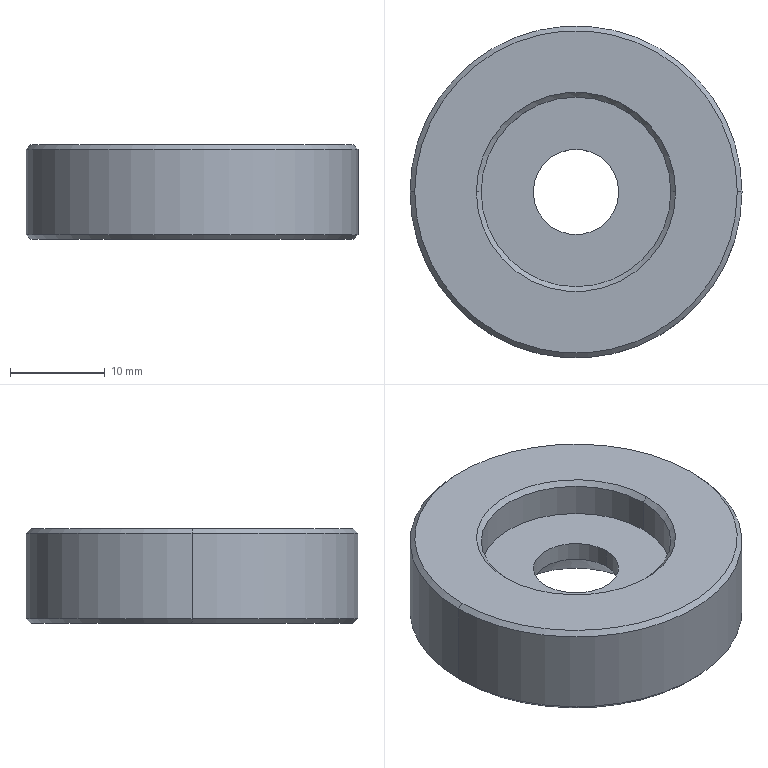Part | SolidWorks | features Chamfer 2, Extrusion 1, HoleWzd 1, ICE 1 | 1 solid | 17 faces | box 35 x 35 x 10 mm | volume 7654 mm3 | cone 8 | cylinder 6 | plane 3 | commonest cylinder face diameters 9 x2 20 x2 35 x2
STEP:
#1=CARTESIAN_POINT('',(-10.,0.,9.5));
#2=VERTEX_POINT('',#1);
#3=CARTESIAN_POINT('',(10.,0.,9.5));
#4=VERTEX_POINT('',#3);
#5=CARTESIAN_POINT('',(0.,0.,9.5));
#6=DIRECTION('',(0.,0.,1.));
#7=DIRECTION('',(1.,0.,0.));
#8=AXIS2_PLACEMENT_3D('',#5,#6,#7);
#9=CIRCLE('',#8,10.);
#10=EDGE_CURVE('',#2,#4,#9,.T.);
#11=ORIENTED_EDGE('',*,*,#10,.F.);
#12=CARTESIAN_POINT('',(-10.5,0.,10.));
#13=VERTEX_POINT('',#12);
#14=CARTESIAN_POINT('',(-10.,0.,9.5));
#15=DIRECTION('',(-0.7071,0.,0.7071));
#16=VECTOR('',#15,1000.);
#17=LINE('',#14,#16);
#18=EDGE_CURVE('',#2,#13,#17,.T.);
#19=ORIENTED_EDGE('',*,*,#18,.T.);
#20=CARTESIAN_POINT('',(10.5,0.,10.));
#21=VERTEX_POINT('',#20);
#22=CARTESIAN_POINT('',(0.,0.,10.));
#23=DIRECTION('',(0.,0.,-1.));
#24=DIRECTION('',(1.,0.,0.));
#25=AXIS2_PLACEMENT_3D('',#22,#23,#24);
#26=CIRCLE('',#25,10.5);
#27=EDGE_CURVE('',#21,#13,#26,.T.);
#28=ORIENTED_EDGE('',*,*,#27,.F.);
#29=CARTESIAN_POINT('',(10.,0.,9.5));
#30=DIRECTION('',(0.7071,0.,0.7071));
#31=VECTOR('',#30,1000.);
#32=LINE('',#29,#31);
#33=EDGE_CURVE('',#4,#21,#32,.T.);
#34=ORIENTED_EDGE('',*,*,#33,.F.);
#35=EDGE_LOOP('',(#11,#19,#28,#34));
#36=FACE_OUTER_BOUND('',#35,.T.);
#37=CARTESIAN_POINT('',(0.,0.,9.5));
#38=DIRECTION('',(0.,0.,1.));
#39=DIRECTION('',(1.,0.,0.));
#40=AXIS2_PLACEMENT_3D('',#37,#38,#39);
#41=CONICAL_SURFACE('',#40,10.,0.7854);
#42=ADVANCED_FACE('',(#36),#41,.F.);
#43=CARTESIAN_POINT('',(-10.,0.,6.));
#44=VERTEX_POINT('',#43);
#45=CARTESIAN_POINT('',(10.,0.,6.));
#46=VERTEX_POINT('',#45);
#47=CARTESIAN_POINT('',(0.,0.,6.));
#48=DIRECTION('',(0.,0.,1.));
#49=DIRECTION('',(1.,0.,0.));
#50=AXIS2_PLACEMENT_3D('',#47,#48,#49);
#51=CIRCLE('',#50,10.);
#52=EDGE_CURVE('',#44,#46,#51,.T.);
#53=ORIENTED_EDGE('',*,*,#52,.F.);
#54=CARTESIAN_POINT('',(-10.,0.,6.));
#55=DIRECTION('',(0.,0.,1.));
#56=VECTOR('',#55,1000.);
#57=LINE('',#54,#56);
#58=EDGE_CURVE('',#44,#2,#57,.T.);
#59=ORIENTED_EDGE('',*,*,#58,.T.);
#60=ORIENTED_EDGE('',*,*,#10,.T.);
#61=CARTESIAN_POINT('',(10.,0.,6.));
#62=DIRECTION('',(0.,0.,1.));
#63=VECTOR('',#62,1000.);
#64=LINE('',#61,#63);
#65=EDGE_CURVE('',#46,#4,#64,.T.);
#66=ORIENTED_EDGE('',*,*,#65,.F.);
#67=EDGE_LOOP('',(#53,#59,#60,#66));
#68=FACE_OUTER_BOUND('',#67,.T.);
#69=CARTESIAN_POINT('',(0.,0.,6.));
#70=DIRECTION('',(0.,0.,1.));
#71=DIRECTION('',(1.,0.,0.));
#72=AXIS2_PLACEMENT_3D('',#69,#70,#71);
#73=CYLINDRICAL_SURFACE('',#72,10.);
#74=ADVANCED_FACE('',(#68),#73,.F.);
#75=CARTESIAN_POINT('',(4.5,0.,4.));
#76=VERTEX_POINT('',#75);
#77=CARTESIAN_POINT('',(-4.5,0.,4.));
#78=VERTEX_POINT('',#77);
#79=CARTESIAN_POINT('',(0.,0.,4.));
#80=DIRECTION('',(0.,0.,-1.));
#81=DIRECTION('',(-1.,0.,0.));
#82=AXIS2_PLACEMENT_3D('',#79,#80,#81);
#83=CIRCLE('',#82,4.5);
#84=EDGE_CURVE('',#76,#78,#83,.T.);
#85=ORIENTED_EDGE('',*,*,#84,.F.);
#86=CARTESIAN_POINT('',(8.5,0.,0.));
#87=VERTEX_POINT('',#86);
#88=CARTESIAN_POINT('',(8.5,0.,0.));
#89=DIRECTION('',(0.7071,0.,-0.7071));
#90=VECTOR('',#89,1000.);
#91=LINE('',#88,#90);
#92=EDGE_CURVE('',#76,#87,#91,.T.);
#93=ORIENTED_EDGE('',*,*,#92,.T.);
#94=CARTESIAN_POINT('',(-8.5,0.,0.));
#95=VERTEX_POINT('',#94);
#96=CARTESIAN_POINT('',(0.,0.,0.));
#97=DIRECTION('',(0.,0.,-1.));
#98=DIRECTION('',(-1.,0.,0.));
#99=AXIS2_PLACEMENT_3D('',#96,#97,#98);
#100=CIRCLE('',#99,8.5);
#101=EDGE_CURVE('',#87,#95,#100,.T.);
#102=ORIENTED_EDGE('',*,*,#101,.T.);
#103=CARTESIAN_POINT('',(-8.5,0.,0.));
#104=DIRECTION('',(-0.7071,0.,-0.7071));
#105=VECTOR('',#104,1000.);
#106=LINE('',#103,#105);
#107=EDGE_CURVE('',#78,#95,#106,.T.);
#108=ORIENTED_EDGE('',*,*,#107,.F.);
#109=EDGE_LOOP('',(#85,#93,#102,#108));
#110=FACE_OUTER_BOUND('',#109,.T.);
#111=CARTESIAN_POINT('',(0.,0.,0.));
#112=DIRECTION('',(0.,0.,-1.));
#113=DIRECTION('',(-1.,0.,0.));
#114=AXIS2_PLACEMENT_3D('',#111,#112,#113);
#115=CONICAL_SURFACE('',#114,8.5,0.7854);
#116=ADVANCED_FACE('',(#110),#115,.F.);
#117=CARTESIAN_POINT('',(-17.,0.,0.));
#118=VERTEX_POINT('',#117);
#119=CARTESIAN_POINT('',(17.,0.,0.));
#120=VERTEX_POINT('',#119);
#121=CARTESIAN_POINT('',(0.,0.,0.));
#122=DIRECTION('',(0.,0.,-1.));
#123=DIRECTION('',(1.,0.,0.));
#124=AXIS2_PLACEMENT_3D('',#121,#122,#123);
#125=CIRCLE('',#124,17.);
#126=EDGE_CURVE('',#118,#120,#125,.T.);
#127=ORIENTED_EDGE('',*,*,#126,.F.);
#128=CARTESIAN_POINT('',(-17.5,0.,0.5));
#129=VERTEX_POINT('',#128);
#130=CARTESIAN_POINT('',(-17.5,0.,0.5));
#131=DIRECTION('',(-0.7071,0.,0.7071));
#132=VECTOR('',#131,1000.);
#133=LINE('',#130,#132);
#134=EDGE_CURVE('',#118,#129,#133,.T.);
#135=ORIENTED_EDGE('',*,*,#134,.T.);
#136=CARTESIAN_POINT('',(17.5,0.,0.5));
#137=VERTEX_POINT('',#136);
#138=CARTESIAN_POINT('',(0.,0.,0.5));
#139=DIRECTION('',(0.,0.,1.));
#140=DIRECTION('',(1.,0.,0.));
#141=AXIS2_PLACEMENT_3D('',#138,#139,#140);
#142=CIRCLE('',#141,17.5);
#143=EDGE_CURVE('',#137,#129,#142,.T.);
#144=ORIENTED_EDGE('',*,*,#143,.F.);
#145=CARTESIAN_POINT('',(17.5,0.,0.5));
#146=DIRECTION('',(0.7071,0.,0.7071));
#147=VECTOR('',#146,1000.);
#148=LINE('',#145,#147);
#149=EDGE_CURVE('',#120,#137,#148,.T.);
#150=ORIENTED_EDGE('',*,*,#149,.F.);
#151=EDGE_LOOP('',(#127,#135,#144,#150));
#152=FACE_OUTER_BOUND('',#151,.T.);
#153=CARTESIAN_POINT('',(0.,0.,0.5));
#154=DIRECTION('',(0.,0.,1.));
#155=DIRECTION('',(1.,0.,0.));
#156=AXIS2_PLACEMENT_3D('',#153,#154,#155);
#157=CONICAL_SURFACE('',#156,17.5,0.7854);
#158=ADVANCED_FACE('',(#152),#157,.T.);
#159=CARTESIAN_POINT('',(17.,0.,10.));
#160=VERTEX_POINT('',#159);
#161=CARTESIAN_POINT('',(-17.,0.,10.));
#162=VERTEX_POINT('',#161);
#163=CARTESIAN_POINT('',(0.,0.,10.));
#164=DIRECTION('',(0.,0.,1.));
#165=DIRECTION('',(1.,0.,0.));
#166=AXIS2_PLACEMENT_3D('',#163,#164,#165);
#167=CIRCLE('',#166,17.);
#168=EDGE_CURVE('',#160,#162,#167,.T.);
#169=ORIENTED_EDGE('',*,*,#168,.F.);
#170=CARTESIAN_POINT('',(17.5,0.,9.5));
#171=VERTEX_POINT('',#170);
#172=CARTESIAN_POINT('',(17.,0.,10.));
#173=DIRECTION('',(0.7071,0.,-0.7071));
#174=VECTOR('',#173,1000.);
#175=LINE('',#172,#174);
#176=EDGE_CURVE('',#160,#171,#175,.T.);
#177=ORIENTED_EDGE('',*,*,#176,.T.);
#178=CARTESIAN_POINT('',(-17.5,0.,9.5));
#179=VERTEX_POINT('',#178);
#180=CARTESIAN_POINT('',(0.,0.,9.5));
#181=DIRECTION('',(0.,0.,-1.));
#182=DIRECTION('',(1.,0.,0.));
#183=AXIS2_PLACEMENT_3D('',#180,#181,#182);
#184=CIRCLE('',#183,17.5);
#185=EDGE_CURVE('',#179,#171,#184,.T.);
#186=ORIENTED_EDGE('',*,*,#185,.F.);
#187=CARTESIAN_POINT('',(-17.,0.,10.));
#188=DIRECTION('',(-0.7071,0.,-0.7071));
#189=VECTOR('',#188,1000.);
#190=LINE('',#187,#189);
#191=EDGE_CURVE('',#162,#179,#190,.T.);
#192=ORIENTED_EDGE('',*,*,#191,.F.);
#193=EDGE_LOOP('',(#169,#177,#186,#192));
#194=FACE_OUTER_BOUND('',#193,.T.);
#195=CARTESIAN_POINT('',(0.,0.,10.));
#196=DIRECTION('',(0.,0.,-1.));
#197=DIRECTION('',(-1.,0.,0.));
#198=AXIS2_PLACEMENT_3D('',#195,#196,#197);
#199=CONICAL_SURFACE('',#198,17.,0.7854);
#200=ADVANCED_FACE('',(#194),#199,.T.);
#201=ORIENTED_EDGE('',*,*,#185,.T.);
#202=CARTESIAN_POINT('',(17.5,0.,10.));
#203=DIRECTION('',(0.,0.,-1.));
#204=VECTOR('',#203,1000.);
#205=LINE('',#202,#204);
#206=EDGE_CURVE('',#171,#137,#205,.T.);
#207=ORIENTED_EDGE('',*,*,#206,.T.);
#208=ORIENTED_EDGE('',*,*,#143,.T.);
#209=CARTESIAN_POINT('',(-17.5,0.,10.));
#210=DIRECTION('',(0.,0.,-1.));
#211=VECTOR('',#210,1000.);
#212=LINE('',#209,#211);
#213=EDGE_CURVE('',#179,#129,#212,.T.);
#214=ORIENTED_EDGE('',*,*,#213,.F.);
#215=EDGE_LOOP('',(#201,#207,#208,#214));
#216=FACE_OUTER_BOUND('',#215,.T.);
#217=CARTESIAN_POINT('',(0.,0.,10.));
#218=DIRECTION('',(0.,0.,-1.));
#219=DIRECTION('',(-1.,0.,0.));
#220=AXIS2_PLACEMENT_3D('',#217,#218,#219);
#221=CYLINDRICAL_SURFACE('',#220,17.5);
#222=ADVANCED_FACE('',(#216),#221,.T.);
#223=CARTESIAN_POINT('',(4.5,0.,6.));
#224=VERTEX_POINT('',#223);
#225=CARTESIAN_POINT('',(-4.5,0.,6.));
#226=VERTEX_POINT('',#225);
#227=CARTESIAN_POINT('',(0.,0.,6.));
#228=DIRECTION('',(0.,0.,-1.));
#229=DIRECTION('',(1.,0.,0.));
#230=AXIS2_PLACEMENT_3D('',#227,#228,#229);
#231=CIRCLE('',#230,4.5);
#232=EDGE_CURVE('',#224,#226,#231,.T.);
#233=ORIENTED_EDGE('',*,*,#232,.F.);
#234=CARTESIAN_POINT('',(4.5,0.,0.));
#235=DIRECTION('',(0.,0.,-1.));
#236=VECTOR('',#235,1000.);
#237=LINE('',#234,#236);
#238=EDGE_CURVE('',#224,#76,#237,.T.);
#239=ORIENTED_EDGE('',*,*,#238,.T.);
#240=ORIENTED_EDGE('',*,*,#84,.T.);
#241=CARTESIAN_POINT('',(-4.5,0.,0.));
#242=DIRECTION('',(0.,0.,-1.));
#243=VECTOR('',#242,1000.);
#244=LINE('',#241,#243);
#245=EDGE_CURVE('',#226,#78,#244,.T.);
#246=ORIENTED_EDGE('',*,*,#245,.F.);
#247=EDGE_LOOP('',(#233,#239,#240,#246));
#248=FACE_OUTER_BOUND('',#247,.T.);
#249=CARTESIAN_POINT('',(0.,0.,0.));
#250=DIRECTION('',(0.,0.,-1.));
#251=DIRECTION('',(-1.,0.,0.));
#252=AXIS2_PLACEMENT_3D('',#249,#250,#251);
#253=CYLINDRICAL_SURFACE('',#252,4.5);
#254=ADVANCED_FACE('',(#248),#253,.F.);
#255=ORIENTED_EDGE('',*,*,#238,.F.);
#256=CARTESIAN_POINT('',(0.,0.,6.));
#257=DIRECTION('',(0.,0.,-1.));
#258=DIRECTION('',(1.,0.,0.));
#259=AXIS2_PLACEMENT_3D('',#256,#257,#258);
#260=CIRCLE('',#259,4.5);
#261=EDGE_CURVE('',#226,#224,#260,.T.);
#262=ORIENTED_EDGE('',*,*,#261,.F.);
#263=ORIENTED_EDGE('',*,*,#245,.T.);
#264=CARTESIAN_POINT('',(0.,0.,4.));
#265=DIRECTION('',(0.,0.,-1.));
#266=DIRECTION('',(-1.,0.,0.));
#267=AXIS2_PLACEMENT_3D('',#264,#265,#266);
#268=CIRCLE('',#267,4.5);
#269=EDGE_CURVE('',#78,#76,#268,.T.);
#270=ORIENTED_EDGE('',*,*,#269,.T.);
#271=EDGE_LOOP('',(#255,#262,#263,#270));
#272=FACE_OUTER_BOUND('',#271,.T.);
#273=CARTESIAN_POINT('',(0.,0.,0.));
#274=DIRECTION('',(0.,0.,-1.));
#275=DIRECTION('',(-1.,0.,0.));
#276=AXIS2_PLACEMENT_3D('',#273,#274,#275);
#277=CYLINDRICAL_SURFACE('',#276,4.5);
#278=ADVANCED_FACE('',(#272),#277,.F.);
#279=ORIENTED_EDGE('',*,*,#206,.F.);
#280=CARTESIAN_POINT('',(0.,0.,9.5));
#281=DIRECTION('',(0.,0.,-1.));
#282=DIRECTION('',(1.,0.,0.));
#283=AXIS2_PLACEMENT_3D('',#280,#281,#282);
#284=CIRCLE('',#283,17.5);
#285=EDGE_CURVE('',#171,#179,#284,.T.);
#286=ORIENTED_EDGE('',*,*,#285,.T.);
#287=ORIENTED_EDGE('',*,*,#213,.T.);
#288=CARTESIAN_POINT('',(0.,0.,0.5));
#289=DIRECTION('',(0.,0.,1.));
#290=DIRECTION('',(1.,0.,0.));
#291=AXIS2_PLACEMENT_3D('',#288,#289,#290);
#292=CIRCLE('',#291,17.5);
#293=EDGE_CURVE('',#129,#137,#292,.T.);
#294=ORIENTED_EDGE('',*,*,#293,.T.);
#295=EDGE_LOOP('',(#279,#286,#287,#294));
#296=FACE_OUTER_BOUND('',#295,.T.);
#297=CARTESIAN_POINT('',(0.,0.,10.));
#298=DIRECTION('',(0.,0.,-1.));
#299=DIRECTION('',(-1.,0.,0.));
#300=AXIS2_PLACEMENT_3D('',#297,#298,#299);
#301=CYLINDRICAL_SURFACE('',#300,17.5);
#302=ADVANCED_FACE('',(#296),#301,.T.);
#303=ORIENTED_EDGE('',*,*,#27,.T.);
#304=CARTESIAN_POINT('',(0.,0.,10.));
#305=DIRECTION('',(0.,0.,-1.));
#306=DIRECTION('',(1.,0.,0.));
#307=AXIS2_PLACEMENT_3D('',#304,#305,#306);
#308=CIRCLE('',#307,10.5);
#309=EDGE_CURVE('',#13,#21,#308,.T.);
#310=ORIENTED_EDGE('',*,*,#309,.T.);
#311=EDGE_LOOP('',(#303,#310));
#312=FACE_BOUND('',#311,.T.);
#313=CARTESIAN_POINT('',(0.,0.,10.));
#314=DIRECTION('',(0.,0.,1.));
#315=DIRECTION('',(1.,0.,0.));
#316=AXIS2_PLACEMENT_3D('',#313,#314,#315);
#317=CIRCLE('',#316,17.);
#318=EDGE_CURVE('',#162,#160,#317,.T.);
#319=ORIENTED_EDGE('',*,*,#318,.T.);
#320=ORIENTED_EDGE('',*,*,#168,.T.);
#321=EDGE_LOOP('',(#319,#320));
#322=FACE_OUTER_BOUND('',#321,.T.);
#323=CARTESIAN_POINT('',(0.,0.,10.));
#324=DIRECTION('',(0.,0.,1.));
#325=DIRECTION('',(1.,0.,0.));
#326=AXIS2_PLACEMENT_3D('',#323,#324,#325);
#327=PLANE('',#326);
#328=ADVANCED_FACE('',(#312,#322),#327,.T.);
#329=CARTESIAN_POINT('',(0.,0.,0.));
#330=DIRECTION('',(0.,0.,-1.));
#331=DIRECTION('',(-1.,0.,0.));
#332=AXIS2_PLACEMENT_3D('',#329,#330,#331);
#333=CIRCLE('',#332,8.5);
#334=EDGE_CURVE('',#95,#87,#333,.T.);
#335=ORIENTED_EDGE('',*,*,#334,.F.);
#336=ORIENTED_EDGE('',*,*,#101,.F.);
#337=EDGE_LOOP('',(#335,#336));
#338=FACE_BOUND('',#337,.T.);
#339=CARTESIAN_POINT('',(0.,0.,0.));
#340=DIRECTION('',(0.,0.,-1.));
#341=DIRECTION('',(1.,0.,0.));
#342=AXIS2_PLACEMENT_3D('',#339,#340,#341);
#343=CIRCLE('',#342,17.);
#344=EDGE_CURVE('',#120,#118,#343,.T.);
#345=ORIENTED_EDGE('',*,*,#344,.T.);
#346=ORIENTED_EDGE('',*,*,#126,.T.);
#347=EDGE_LOOP('',(#345,#346));
#348=FACE_OUTER_BOUND('',#347,.T.);
#349=CARTESIAN_POINT('',(0.,0.,0.));
#350=DIRECTION('',(0.,0.,1.));
#351=DIRECTION('',(1.,0.,0.));
#352=AXIS2_PLACEMENT_3D('',#349,#350,#351);
#353=PLANE('',#352);
#354=ADVANCED_FACE('',(#338,#348),#353,.F.);
#355=ORIENTED_EDGE('',*,*,#176,.F.);
#356=ORIENTED_EDGE('',*,*,#318,.F.);
#357=ORIENTED_EDGE('',*,*,#191,.T.);
#358=ORIENTED_EDGE('',*,*,#285,.F.);
#359=EDGE_LOOP('',(#355,#356,#357,#358));
#360=FACE_OUTER_BOUND('',#359,.T.);
#361=CARTESIAN_POINT('',(0.,0.,10.));
#362=DIRECTION('',(0.,0.,-1.));
#363=DIRECTION('',(-1.,0.,0.));
#364=AXIS2_PLACEMENT_3D('',#361,#362,#363);
#365=CONICAL_SURFACE('',#364,17.,0.7854);
#366=ADVANCED_FACE('',(#360),#365,.T.);
#367=ORIENTED_EDGE('',*,*,#134,.F.);
#368=ORIENTED_EDGE('',*,*,#344,.F.);
#369=ORIENTED_EDGE('',*,*,#149,.T.);
#370=ORIENTED_EDGE('',*,*,#293,.F.);
#371=EDGE_LOOP('',(#367,#368,#369,#370));
#372=FACE_OUTER_BOUND('',#371,.T.);
#373=CARTESIAN_POINT('',(0.,0.,0.5));
#374=DIRECTION('',(0.,0.,1.));
#375=DIRECTION('',(1.,0.,0.));
#376=AXIS2_PLACEMENT_3D('',#373,#374,#375);
#377=CONICAL_SURFACE('',#376,17.5,0.7854);
#378=ADVANCED_FACE('',(#372),#377,.T.);
#379=ORIENTED_EDGE('',*,*,#92,.F.);
#380=ORIENTED_EDGE('',*,*,#269,.F.);
#381=ORIENTED_EDGE('',*,*,#107,.T.);
#382=ORIENTED_EDGE('',*,*,#334,.T.);
#383=EDGE_LOOP('',(#379,#380,#381,#382));
#384=FACE_OUTER_BOUND('',#383,.T.);
#385=CARTESIAN_POINT('',(0.,0.,0.));
#386=DIRECTION('',(0.,0.,-1.));
#387=DIRECTION('',(-1.,0.,0.));
#388=AXIS2_PLACEMENT_3D('',#385,#386,#387);
#389=CONICAL_SURFACE('',#388,8.5,0.7854);
#390=ADVANCED_FACE('',(#384),#389,.F.);
#391=CARTESIAN_POINT('',(0.,0.,6.));
#392=DIRECTION('',(0.,0.,1.));
#393=DIRECTION('',(1.,0.,0.));
#394=AXIS2_PLACEMENT_3D('',#391,#392,#393);
#395=CIRCLE('',#394,10.);
#396=EDGE_CURVE('',#46,#44,#395,.T.);
#397=ORIENTED_EDGE('',*,*,#396,.T.);
#398=ORIENTED_EDGE('',*,*,#52,.T.);
#399=EDGE_LOOP('',(#397,#398));
#400=FACE_OUTER_BOUND('',#399,.T.);
#401=ORIENTED_EDGE('',*,*,#261,.T.);
#402=ORIENTED_EDGE('',*,*,#232,.T.);
#403=EDGE_LOOP('',(#401,#402));
#404=FACE_BOUND('',#403,.T.);
#405=CARTESIAN_POINT('',(0.,0.,6.));
#406=DIRECTION('',(0.,0.,1.));
#407=DIRECTION('',(1.,0.,0.));
#408=AXIS2_PLACEMENT_3D('',#405,#406,#407);
#409=PLANE('',#408);
#410=ADVANCED_FACE('',(#400,#404),#409,.T.);
#411=ORIENTED_EDGE('',*,*,#58,.F.);
#412=ORIENTED_EDGE('',*,*,#396,.F.);
#413=ORIENTED_EDGE('',*,*,#65,.T.);
#414=CARTESIAN_POINT('',(0.,0.,9.5));
#415=DIRECTION('',(0.,0.,1.));
#416=DIRECTION('',(1.,0.,0.));
#417=AXIS2_PLACEMENT_3D('',#414,#415,#416);
#418=CIRCLE('',#417,10.);
#419=EDGE_CURVE('',#4,#2,#418,.T.);
#420=ORIENTED_EDGE('',*,*,#419,.T.);
#421=EDGE_LOOP('',(#411,#412,#413,#420));
#422=FACE_OUTER_BOUND('',#421,.T.);
#423=CARTESIAN_POINT('',(0.,0.,6.));
#424=DIRECTION('',(0.,0.,1.));
#425=DIRECTION('',(1.,0.,0.));
#426=AXIS2_PLACEMENT_3D('',#423,#424,#425);
#427=CYLINDRICAL_SURFACE('',#426,10.);
#428=ADVANCED_FACE('',(#422),#427,.F.);
#429=ORIENTED_EDGE('',*,*,#18,.F.);
#430=ORIENTED_EDGE('',*,*,#419,.F.);
#431=ORIENTED_EDGE('',*,*,#33,.T.);
#432=ORIENTED_EDGE('',*,*,#309,.F.);
#433=EDGE_LOOP('',(#429,#430,#431,#432));
#434=FACE_OUTER_BOUND('',#433,.T.);
#435=CARTESIAN_POINT('',(0.,0.,9.5));
#436=DIRECTION('',(0.,0.,1.));
#437=DIRECTION('',(1.,0.,0.));
#438=AXIS2_PLACEMENT_3D('',#435,#436,#437);
#439=CONICAL_SURFACE('',#438,10.,0.7854);
#440=ADVANCED_FACE('',(#434),#439,.F.);
#441=CLOSED_SHELL('',(#42,#74,#116,#158,#200,#222,#254,#278,#302,#328,#354,#366,#378,#390,#410,#428,#440));
#442=MANIFOLD_SOLID_BREP('',#441);
#443=CARTESIAN_POINT('',(0.,0.,0.));
#444=DIRECTION('',(0.,0.,1.));
#445=DIRECTION('',(1.,0.,0.));
#446=AXIS2_PLACEMENT_3D('',#443,#444,#445);
#447=(LENGTH_UNIT()NAMED_UNIT(*)SI_UNIT(.MILLI.,.METRE.));
#448=UNCERTAINTY_MEASURE_WITH_UNIT(LENGTH_MEASURE(0.00001),#447,'','');
#449=(NAMED_UNIT(*)PLANE_ANGLE_UNIT()SI_UNIT($,.RADIAN.));
#450=(NAMED_UNIT(*)SI_UNIT($,.STERADIAN.)SOLID_ANGLE_UNIT());
#451=(GEOMETRIC_REPRESENTATION_CONTEXT(3)GLOBAL_UNCERTAINTY_ASSIGNED_CONTEXT((#448))GLOBAL_UNIT_ASSIGNED_CONTEXT((#447,#449,#450))REPRESENTATION_CONTEXT('',''));
#452=ADVANCED_BREP_SHAPE_REPRESENTATION('',(#442,#446),#451);